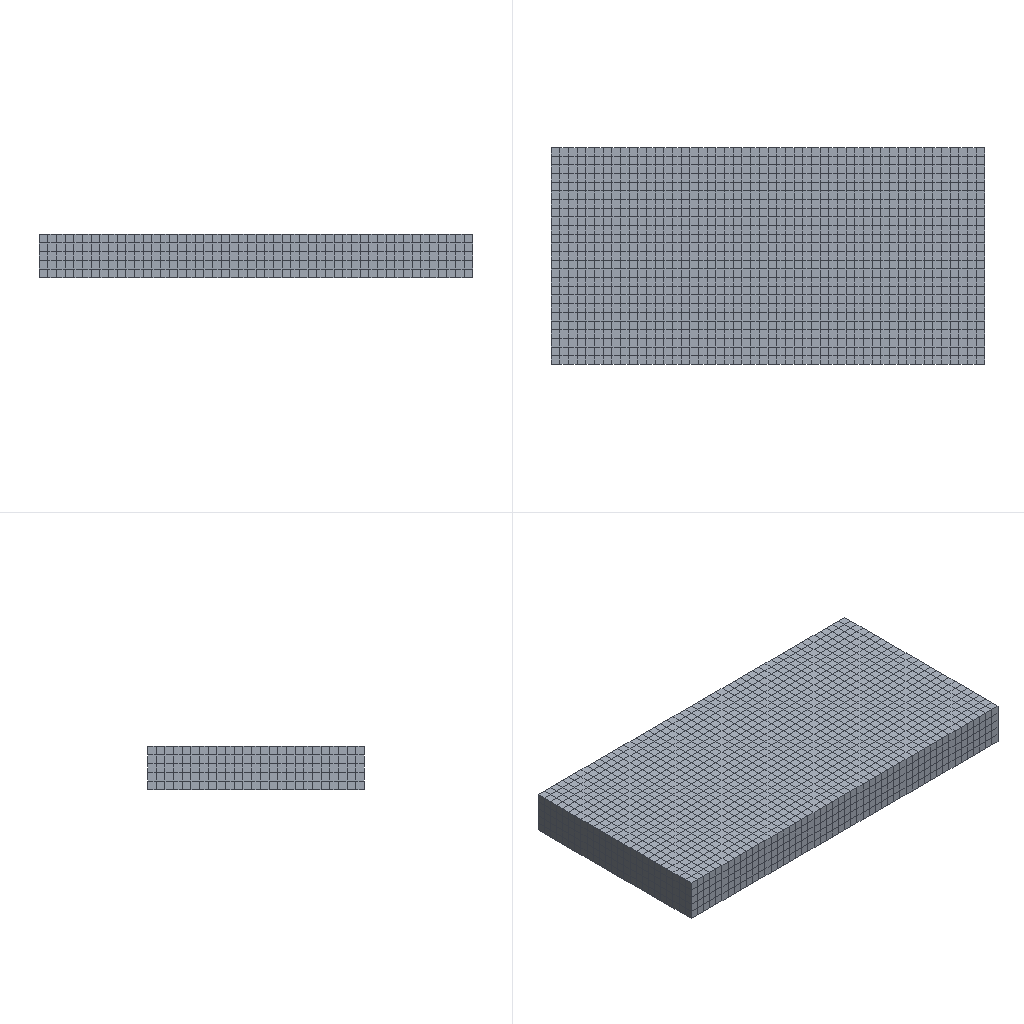Simulation study | abaqus
Abaqus input file, long lists of numbers shortened:
*Heading
** Job name: deck-1 Model name: Model-1
** Generated by: Abaqus/CAE 2024
*Preprint, echo=NO, model=NO, history=NO, contact=NO
**
** PARTS
**
*Part, name=Part-1
*Node
      1,           0.,         -25.,           5.
      2,           0.,         -24.,           5.
** (7954 more lines like these left out)
*Element, type=C3D8R
   1,  157,  158,  184,  183,    1,    2,   28,   27
   2,  158,  159,  185,  184,    2,    3,   29,   28
** (6248 more lines like these left out)
*Nset, nset=Set-1, generate
    1,  7956,     1
*Elset, elset=Set-1, generate
    1,  6250,     1
** Section: Section-1
*Solid Section, elset=Set-1, material=Material-1
,
*End Part
**
*Part, name=tool
*Node
      1,           5.,         10.5,           2.
      2,           5.,   3.762,           2.
** (472 more lines like these left out)
*Element, type=R3D4
 1,   1,   9, 109,  40
 2,   9,  10, 110, 109
** (470 more lines like these left out)
*Node
    475,           5.,         10.5,           1.
*Nset, nset=tool-RefPt_, internal
475,
*Elset, elset=tool, generate
   1,  472,    1
*End Part
**
**
** ASSEMBLY
**
*Assembly, name=Assembly
**
*Instance, name=Part-1-1, part=Part-1
*End Instance
**
*Instance, name=tool-1, part=tool
         50.,        -11.5,          0.5
         50.,        -11.5,          0.5, 51.,        -11.5,          0.5, 90.
*End Instance
**
*Instance, name=tool-1-lin-2-1, part=tool
         50.,         -5.5,          0.5
         50.,         -5.5,          0.5, 51.,         -5.5,          0.5, 90.
*End Instance
**
*Instance, name=tool-1-lin-2-1-1, part=tool
         50.,        -17.5,          0.5
         50.,        -17.5,          0.5, 51.,        -17.5,          0.5, 90.
*End Instance
**
*Nset, nset=Set-1, instance=Part-1-1
  131,  132,  133,  134,  135,  136,  137,  138,  139,  140,  141,  142,  143,  144,  145,  146
  147,  148,  149,  150,  151,  152,  153,  154,  155,  156,  287,  288,  289,  290,  291,  292
** (81 more lines like these left out)
*Elset, elset=Set-1, instance=Part-1-1
  101,  102,  103,  104,  105,  106,  107,  108,  109,  110,  111,  112,  113,  114,  115,  116
  117,  118,  119,  120,  121,  122,  123,  124,  125,  226,  227,  228,  229,  230,  231,  232
** (77 more lines like these left out)
*Nset, nset=Set-3, instance=tool-1-lin-2-1-1
 475,
*Nset, nset=Set-4, instance=tool-1
 475,
*Nset, nset=Set-5, instance=tool-1-lin-2-1
 475,
*Nset, nset=s_Set-2, instance=Part-1-1, generate
    1,  7956,     1
*Elset, elset=s_Set-2, instance=Part-1-1, generate
    1,  6250,     1
*Elset, elset=_m_Surf-1_SPOS, internal, instance=tool-1-lin-2-1-1, generate
   1,  472,    1
*Surface, type=ELEMENT, name=m_Surf-1
_m_Surf-1_SPOS, SPOS
*Elset, elset=_m_Surf-2_SPOS, internal, instance=tool-1, generate
   1,  472,    1
*Surface, type=ELEMENT, name=m_Surf-2
_m_Surf-2_SPOS, SPOS
*Elset, elset=_m_Surf-3_SPOS, internal, instance=tool-1-lin-2-1, generate
   1,  472,    1
*Surface, type=ELEMENT, name=m_Surf-3
_m_Surf-3_SPOS, SPOS
*Surface, type=NODE, name=s_Set-2_CNS_, internal
s_Set-2, 1.
*Rigid Body, ref node=tool-1.tool-RefPt_, elset=tool-1.tool
*Rigid Body, ref node=tool-1-lin-2-1.tool-RefPt_, elset=tool-1-lin-2-1.tool
*Rigid Body, ref node=tool-1-lin-2-1-1.tool-RefPt_, elset=tool-1-lin-2-1-1.tool
*End Assembly
**
** MATERIALS
**
*Material, name=Material-1
*Damage Initiation, criterion=SHEAR
 0.1,0.,0.
*Damage Evolution, type=DISPLACEMENT
 1e-05,
*Density
 2.8e-09,
*Elastic
72000., 0.3
*Plastic
200.,0.
**
** INTERACTION PROPERTIES
**
*Surface Interaction, name=IntProp-1
*Friction
 0.2,
*Surface Behavior, pressure-overclosure=HARD
** ----------------------------------------------------------------
**
** STEP: Step-1
**
*Step, name=Step-1, nlgeom=YES
*Dynamic, Explicit
, 0.01
*Bulk Viscosity
0.06, 1.2
** Mass Scaling: Semi-Automatic
**               Whole Model
*Fixed Mass Scaling, factor=500.
**
** BOUNDARY CONDITIONS
**
** Name: BC-fix Type: Symmetry/Antisymmetry/Encastre
*Boundary
Set-1, ENCASTRE
** Name: BC-v1 Type: Velocity/Angular velocity
*Boundary, type=VELOCITY
Set-3, 1, 1, -5600.
Set-3, 2, 2
Set-3, 3, 3
Set-3, 4, 4
Set-3, 5, 5
Set-3, 6, 6
** Name: BC-v2 Type: Velocity/Angular velocity
*Boundary, type=VELOCITY
Set-4, 1, 1
Set-4, 2, 2
Set-4, 3, 3
Set-4, 4, 4
Set-4, 5, 5
Set-4, 6, 6
** Name: BC-v3 Type: Velocity/Angular velocity
*Boundary, type=VELOCITY
Set-5, 1, 1
Set-5, 2, 2
Set-5, 3, 3
Set-5, 4, 4
Set-5, 5, 5
Set-5, 6, 6
**
** INTERACTIONS
**
** Interaction: Int-1
*Contact Pair, interaction=IntProp-1, mechanical constraint=KINEMATIC, cpset=Int-1
m_Surf-1, s_Set-2_CNS_
** Interaction: Int-1-Copy
*Contact Pair, interaction=IntProp-1, mechanical constraint=KINEMATIC, cpset=Int-1-Copy
m_Surf-2, s_Set-2_CNS_
** Interaction: Int-1-Copy2
*Contact Pair, interaction=IntProp-1, mechanical constraint=KINEMATIC, cpset=Int-1-Copy2
m_Surf-3, s_Set-2_CNS_
**
** OUTPUT REQUESTS
**
*Restart, write, number interval=1, time marks=NO
**
** FIELD OUTPUT: F-Output-1
**
*Output, field, number interval=40
*Node Output
A, CF, RF, RM, RT, U, V
*Element Output, directions=YES
E, EVF, LE, MISES, MISESMAX, PE, PEEQ, PEEQVAVG, PEVAVG, S, STATUS, SVAVG
*Contact Output
CDISP, CSTRESS
**
** HISTORY OUTPUT: H-Output-1
**
*Output, history, time interval=2e-07
*Node Output, nset=Set-1
RF1, RF2, RF3
*End Step
** ----------------------------------------------------------------
**
** STEP: Step-2
**
*Step, name=Step-2, nlgeom=YES
*Dynamic, Explicit
, 0.01
*Bulk Viscosity
0.06, 1.2
** Mass Scaling: Semi-Automatic
**               Whole Model
*Fixed Mass Scaling, factor=500.
**
** BOUNDARY CONDITIONS
**
** Name: BC-v1 Type: Velocity/Angular velocity
*Boundary, type=VELOCITY
Set-3, 1, 1
** Name: BC-v2 Type: Velocity/Angular velocity
*Boundary, type=VELOCITY
Set-4, 1, 1, -5600.
**
** OUTPUT REQUESTS
**
*Restart, write, number interval=1, time marks=NO
**
** FIELD OUTPUT: F-Output-1
**
*Output, field, number interval=40
*Node Output
A, CF, RF, RM, RT, U, V
*Element Output, directions=YES
E, EVF, LE, MISES, MISESMAX, PE, PEEQ, PEEQVAVG, PEVAVG, S, STATUS, SVAVG
*Contact Output
CDISP, CSTRESS
**
** HISTORY OUTPUT: H-Output-2
**
*Output, history, time interval=2e-07
*Node Output, nset=Set-3
RF1, RF2, RF3
*End Step
** ----------------------------------------------------------------
**
** STEP: Step-3
**
*Step, name=Step-3, nlgeom=YES
*Dynamic, Explicit
, 0.01
*Bulk Viscosity
0.06, 1.2
** Mass Scaling: Semi-Automatic
**               Whole Model
*Fixed Mass Scaling, factor=500.
**
** BOUNDARY CONDITIONS
**
** Name: BC-v2 Type: Velocity/Angular velocity
*Boundary, type=VELOCITY
Set-4, 1, 1
** Name: BC-v3 Type: Velocity/Angular velocity
*Boundary, type=VELOCITY
Set-5, 1, 1, -5600.
**
** OUTPUT REQUESTS
**
*Restart, write, number interval=1, time marks=NO
**
** FIELD OUTPUT: F-Output-1
**
*Output, field, number interval=40
*Node Output
A, CF, RF, RM, RT, U, V
*Element Output, directions=YES
E, EVF, LE, MISES, MISESMAX, PE, PEEQ, PEEQVAVG, PEVAVG, S, STATUS, SVAVG
*Contact Output
CDISP, CSTRESS
**
** HISTORY OUTPUT: H-Output-3
**
*Output, history, time interval=2e-07
*Node Output, nset=Set-5
RF1, RF2, RF3
*End Step